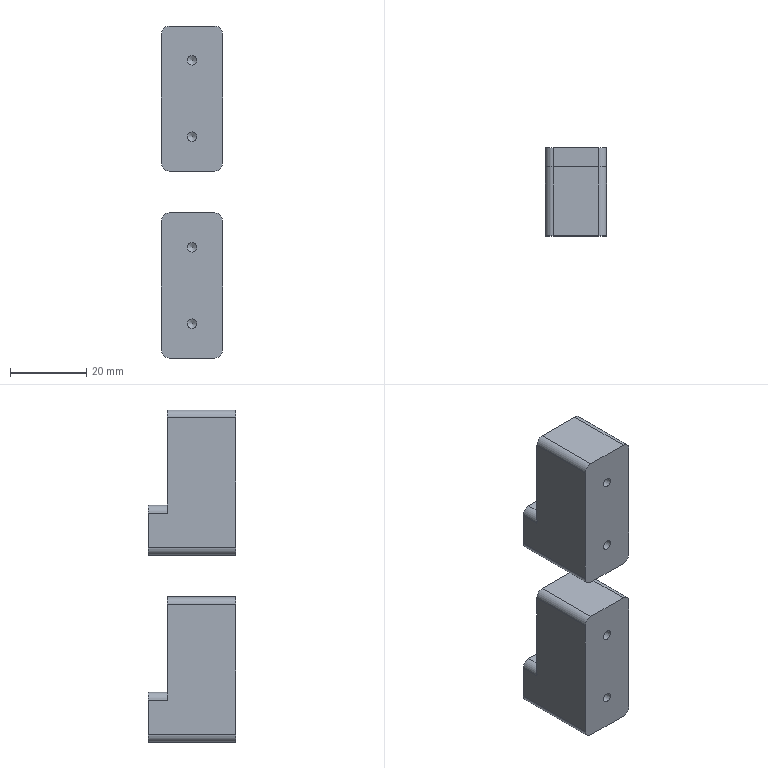CAM job | NX | 3+2 milling, drilling | part box 16 x 23 x 87 mm | stock box 21 x 25 x 92 mm
Tools:
number,name,description,diameter,corner_radius,flute_length,length,flutes
9,D10,平底铣刀-粗,10.0,0.0,35.0,75.0,2
7,D6-J,平底铣刀-精,6.0,0.0,25.0,75.0,2
10,D10-J,平底铣刀-精,10.0,0.0,35.0,75.0,2
1,D80R0.8FACEMILL,圆鼻刀-粗,80.0,0.8,50.0,75.0,2
1,D80R0.8FACEMILL-J,圆鼻刀-精,80.0,0.8,50.0,75.0,2
2,D6CHAMFERMILL,倒角刀,6.0,0.0,3.0,25.0,2
20,M3X0.5,丝锥,2.5,0.0,35.0,50.0,2
21,M4X0.7,丝锥,3.3,0.0,35.0,50.0,2
12,ZT2.5,钻头,2.5,0.0,35.0,50.0,2
13,DRILL3.3,Twist Drill 3.3 mm,3.3,0.0,35.0,35.008,2
Operations:
program,operation,operation_type,tool,method,geometry_group,spindle_rpm,surface_speed,feed_per_tooth,feed_cut,feed_plunge,cut_length_mm,path_length_mm,cut_time_min,machine_time_min
B,FLOORFACEONEROUGH_COPY,VolumeBased25DMillingOperation,D80R0.8FACEMILL,LAYERROUGH-DEPTHK-STEPG,W-B,2800.0,703.696,0.5357,3000.0,100.0,975.97,1809.948,0.3253,0.4087
B,FLOORFACEONEFINISH_COPY,VolumeBased25DMillingOperation,D80R0.8FACEMILL-J,SIDEFINISH-DEPTHK-STEPG,W-B,4000.0,1005.28,0.125,1000.0,100.0,194.998,230.998,0.195,0.1986
B,FLOORLAYERROUGH-MID_COPY,VolumeBased25DMillingOperation,D10,LAYERROUGH-DEPTHK-STEPG,W-B,8000.0,251.32,0.25,4000.0,100.0,2661.738,3248.189,0.6654,0.7241
B,SPOTDRILL-DEPTH0.8_2,Operation,D6CHAMFERMILL,NONE,W-B,8000.0,150.796,0.0312,500.0,90.0,3.6,107.21,0.0072,0.0176
B,BLINDHOLE-M4TAPDRILL,Operation,DRILL3.3,NONE,W-B,3000.0,31.102,0.02,120.0,90.0,24.183,148.376,0.2015,0.2139
B,DRILLCHAMFER_2,Operation,D6CHAMFERMILL,METHOD,W-B,8000.0,150.796,0.0312,500.0,0.0,10.4,122.892,0.0208,0.032
B,FACEDEBURR6X45L_COPY,SurfaceContour,D6CHAMFERMILL,CLIMBCHAMFER-DEPTH0-STEPG,W-B,6500.0,122.519,0.1154,1500.0,100.0,289.393,554.925,0.1929,0.2195
B,BLINDHOLE-TAPM4,Operation,M4X0.7,METHOD,W-B,800.0,8.294,0.0004,0.7,90.0,18.2,136.41,26.0,26.012
B,FLOORFINISHBOTTOM-MID_COPY,VolumeBased25DMillingOperation,D6-J,FINISHSTEPDEPTHOFF,W-B,8000.0,150.792,0.0625,1000.0,100.0,340.807,472.183,0.3408,0.3539
B,FLOORFINISHSIDE-MID-SELBOTTOM_COPY,VolumeBased25DMillingOperation,D6-J,SIDEFINISH-DEPTHK-STEPG,W-B,8000.0,150.792,0.0625,1000.0,100.0,66.912,185.03,0.0669,0.0787
A,TOPFACEROUGH,FaceMilling,D80R0.8FACEMILL,LAYERROUGH-DEPTHK-STEPG,W-A,4000.0,1005.31,0.375,3000.0,100.0,181.0,216.8,0.0603,0.0639
A,TOPFACE,FaceMilling,D80R0.8FACEMILL,SIDEFINISH-DEPTHK-STEPG,W-A,4000.0,1005.31,0.125,1000.0,100.0,181.0,217.0,0.181,0.1846
A,PROFILEROUGH_2,VolumeBased25DMillingOperation,D10,METHOD,W-A,8000.0,251.327,0.3125,5000.0,80.0,13390.925,13563.625,2.678,2.696
A,SPOTDRILL-DEPTH0.8,Operation,D6CHAMFERMILL,NONE,W-A,8000.0,150.796,0.0312,500.0,90.0,7.2,126.467,0.0144,0.0263
A,BLINDHOLE-M3TAPDRILL,Operation,ZT2.5,NONE,W-A,3000.0,23.562,0.0167,100.0,90.0,57.004,226.076,0.57,0.587
A,SELECTBODYONLY,SurfaceContour,D6CHAMFERMILL,METHOD,W-A,8000.0,150.796,0.1875,3000.0,100.0,243.762,363.865,0.0813,0.0933
A,DRILLCHAMFER_1,Operation,D6CHAMFERMILL,METHOD,W-A,8000.0,150.796,0.0312,500.0,0.0,19.0,156.602,0.038,0.0518
A,BLINDHOLE-TAPM3,Operation,M3X0.5,METHOD,W-A,1000.0,7.854,0.0003,0.5,90.0,46.0,204.067,92.0,92.016
A,PROFILESEMI_2,VolumeBased25DMillingOperation,D10-J,METHOD,W-A,8000.0,251.327,0.0625,1000.0,100.0,583.884,739.597,0.5839,0.5995